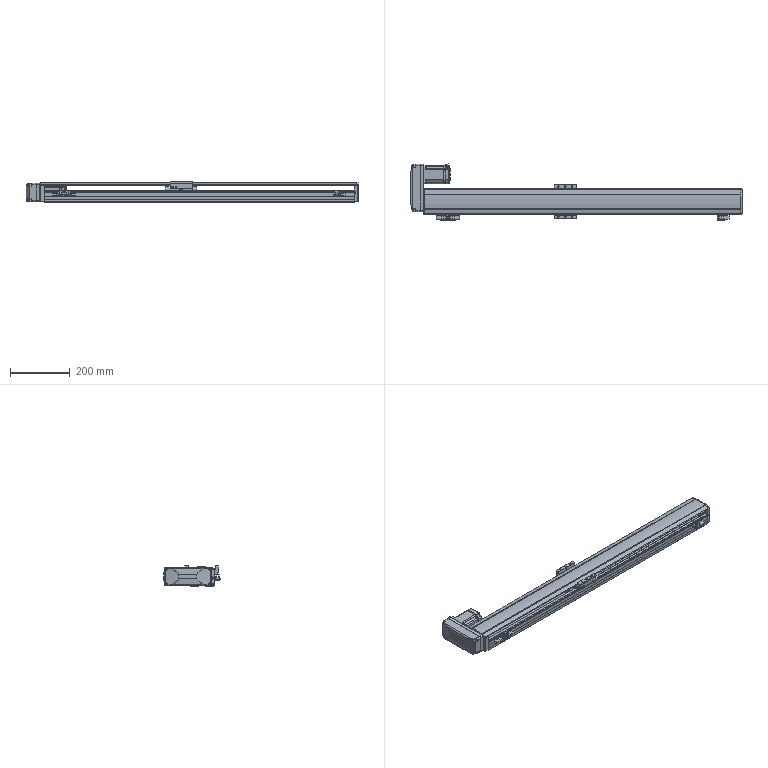Part | SolidWorks | 18 solids | 1560 faces | box 1114 x 188.406 x 68 mm | volume 3201013 mm3 | plane 696 | cylinder 647 | cone 103 | spline 90 | torus 18 | sphere 6 | commonest cylinder face diameters 6 x57 2 x45 2.5 x40 3.3 x40 6.6 x40 11 x40